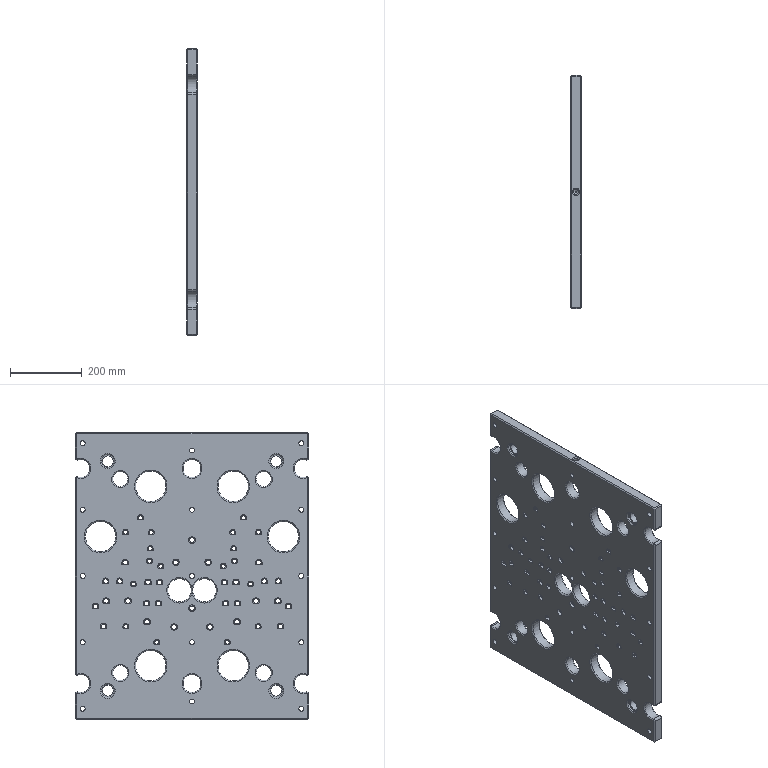Part | STEP file | solid 16 | 1 solid | 429 faces | box 30 x 650 x 800 mm | volume 13444333 mm3 | cylinder 231 | plane 134 | cone 64 | commonest cylinder face diameters 4 x84 13 x30 18 x28 11 x18 16 x18 14 x17